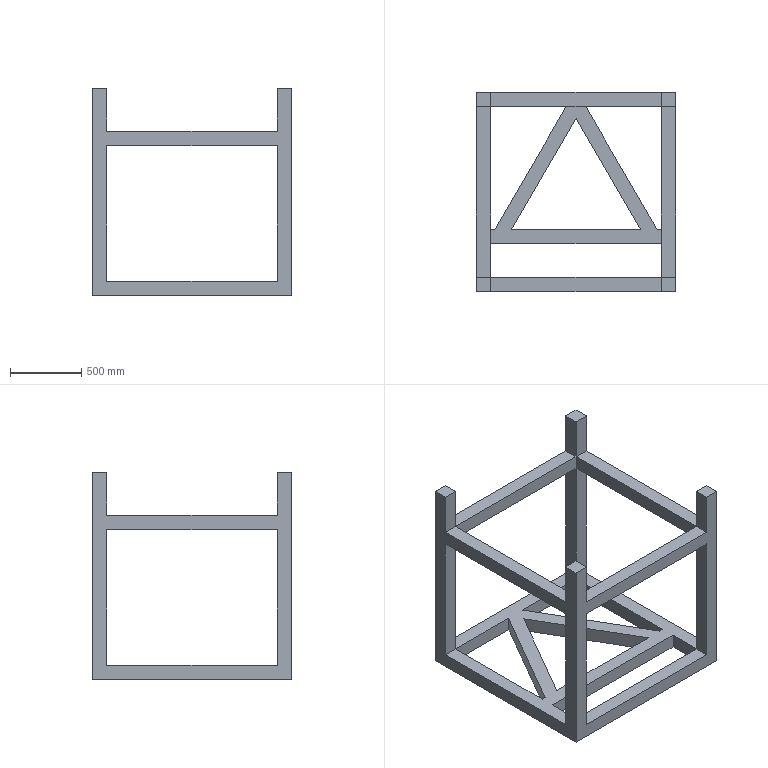Part | SolidWorks | features ICE 3, Extrusion 1 | 1 solid | 54 faces | box 1395 x 1395 x 1450 mm | volume 185057639 mm3 | plane 54
STEP:
#1=CARTESIAN_POINT('',(1395.,1295.,1150.));
#2=VERTEX_POINT('',#1);
#3=CARTESIAN_POINT('',(1295.,1295.,1150.));
#4=VERTEX_POINT('',#3);
#5=CARTESIAN_POINT('',(0.,1295.,1150.));
#6=DIRECTION('',(-1.,0.,0.));
#7=VECTOR('',#6,1000.);
#8=LINE('',#5,#7);
#9=EDGE_CURVE('',#2,#4,#8,.T.);
#10=ORIENTED_EDGE('',*,*,#9,.F.);
#11=CARTESIAN_POINT('',(1395.,1295.,1450.));
#12=VERTEX_POINT('',#11);
#13=CARTESIAN_POINT('',(1395.,1295.,1450.));
#14=DIRECTION('',(0.,0.,-1.));
#15=VECTOR('',#14,1000.);
#16=LINE('',#13,#15);
#17=EDGE_CURVE('',#12,#2,#16,.T.);
#18=ORIENTED_EDGE('',*,*,#17,.F.);
#19=CARTESIAN_POINT('',(1295.,1295.,1450.));
#20=VERTEX_POINT('',#19);
#21=CARTESIAN_POINT('',(1395.,1295.,1450.));
#22=DIRECTION('',(1.,0.,0.));
#23=VECTOR('',#22,1000.);
#24=LINE('',#21,#23);
#25=EDGE_CURVE('',#20,#12,#24,.T.);
#26=ORIENTED_EDGE('',*,*,#25,.F.);
#27=CARTESIAN_POINT('',(1295.,1295.,1450.));
#28=DIRECTION('',(0.,0.,-1.));
#29=VECTOR('',#28,1000.);
#30=LINE('',#27,#29);
#31=EDGE_CURVE('',#20,#4,#30,.T.);
#32=ORIENTED_EDGE('',*,*,#31,.T.);
#33=EDGE_LOOP('',(#10,#18,#26,#32));
#34=FACE_OUTER_BOUND('',#33,.T.);
#35=CARTESIAN_POINT('',(0.,1295.,1450.));
#36=DIRECTION('',(0.,1.,0.));
#37=DIRECTION('',(0.,0.,1.));
#38=AXIS2_PLACEMENT_3D('',#35,#36,#37);
#39=PLANE('',#38);
#40=ADVANCED_FACE('',(#34),#39,.F.);
#41=CARTESIAN_POINT('',(1295.,1295.,1050.));
#42=VERTEX_POINT('',#41);
#43=CARTESIAN_POINT('',(1295.,1295.,1450.));
#44=DIRECTION('',(0.,0.,-1.));
#45=VECTOR('',#44,1000.);
#46=LINE('',#43,#45);
#47=EDGE_CURVE('',#4,#42,#46,.T.);
#48=ORIENTED_EDGE('',*,*,#47,.F.);
#49=CARTESIAN_POINT('',(100.,1295.,1150.));
#50=VERTEX_POINT('',#49);
#51=CARTESIAN_POINT('',(1300.,1295.,1150.));
#52=DIRECTION('',(-1.,0.,0.));
#53=VECTOR('',#52,1000.);
#54=LINE('',#51,#53);
#55=EDGE_CURVE('',#4,#50,#54,.T.);
#56=ORIENTED_EDGE('',*,*,#55,.T.);
#57=CARTESIAN_POINT('',(100.,1295.,1050.));
#58=VERTEX_POINT('',#57);
#59=CARTESIAN_POINT('',(100.,1295.,1450.));
#60=DIRECTION('',(0.,0.,1.));
#61=VECTOR('',#60,1000.);
#62=LINE('',#59,#61);
#63=EDGE_CURVE('',#58,#50,#62,.T.);
#64=ORIENTED_EDGE('',*,*,#63,.F.);
#65=CARTESIAN_POINT('',(1300.,1295.,1050.));
#66=DIRECTION('',(-1.,0.,0.));
#67=VECTOR('',#66,1000.);
#68=LINE('',#65,#67);
#69=EDGE_CURVE('',#42,#58,#68,.T.);
#70=ORIENTED_EDGE('',*,*,#69,.F.);
#71=EDGE_LOOP('',(#48,#56,#64,#70));
#72=FACE_OUTER_BOUND('',#71,.T.);
#73=CARTESIAN_POINT('',(0.,1295.,1450.));
#74=DIRECTION('',(0.,1.,0.));
#75=DIRECTION('',(0.,0.,1.));
#76=AXIS2_PLACEMENT_3D('',#73,#74,#75);
#77=PLANE('',#76);
#78=ADVANCED_FACE('',(#72),#77,.F.);
#79=CARTESIAN_POINT('',(1395.,1295.,1050.));
#80=VERTEX_POINT('',#79);
#81=CARTESIAN_POINT('',(0.,1295.,1050.));
#82=DIRECTION('',(1.,0.,0.));
#83=VECTOR('',#82,1000.);
#84=LINE('',#81,#83);
#85=EDGE_CURVE('',#42,#80,#84,.T.);
#86=ORIENTED_EDGE('',*,*,#85,.F.);
#87=CARTESIAN_POINT('',(1295.,1295.,100.));
#88=VERTEX_POINT('',#87);
#89=CARTESIAN_POINT('',(1295.,1295.,1450.));
#90=DIRECTION('',(0.,0.,-1.));
#91=VECTOR('',#90,1000.);
#92=LINE('',#89,#91);
#93=EDGE_CURVE('',#42,#88,#92,.T.);
#94=ORIENTED_EDGE('',*,*,#93,.T.);
#95=CARTESIAN_POINT('',(1395.,1295.,100.));
#96=VERTEX_POINT('',#95);
#97=CARTESIAN_POINT('',(1395.,1295.,100.));
#98=DIRECTION('',(1.,0.,0.));
#99=VECTOR('',#98,1000.);
#100=LINE('',#97,#99);
#101=EDGE_CURVE('',#88,#96,#100,.T.);
#102=ORIENTED_EDGE('',*,*,#101,.T.);
#103=CARTESIAN_POINT('',(1395.,1295.,1450.));
#104=DIRECTION('',(0.,0.,-1.));
#105=VECTOR('',#104,1000.);
#106=LINE('',#103,#105);
#107=EDGE_CURVE('',#80,#96,#106,.T.);
#108=ORIENTED_EDGE('',*,*,#107,.F.);
#109=EDGE_LOOP('',(#86,#94,#102,#108));
#110=FACE_OUTER_BOUND('',#109,.T.);
#111=CARTESIAN_POINT('',(0.,1295.,1450.));
#112=DIRECTION('',(0.,1.,0.));
#113=DIRECTION('',(0.,0.,1.));
#114=AXIS2_PLACEMENT_3D('',#111,#112,#113);
#115=PLANE('',#114);
#116=ADVANCED_FACE('',(#110),#115,.F.);
#117=CARTESIAN_POINT('',(1295.,100.,1150.));
#118=VERTEX_POINT('',#117);
#119=CARTESIAN_POINT('',(1395.,100.,1150.));
#120=VERTEX_POINT('',#119);
#121=CARTESIAN_POINT('',(1295.,100.,1150.));
#122=DIRECTION('',(1.,0.,0.));
#123=VECTOR('',#122,1000.);
#124=LINE('',#121,#123);
#125=EDGE_CURVE('',#118,#120,#124,.T.);
#126=ORIENTED_EDGE('',*,*,#125,.F.);
#127=CARTESIAN_POINT('',(1295.,100.,1450.));
#128=VERTEX_POINT('',#127);
#129=CARTESIAN_POINT('',(1295.,100.,1450.));
#130=DIRECTION('',(0.,0.,-1.));
#131=VECTOR('',#130,1000.);
#132=LINE('',#129,#131);
#133=EDGE_CURVE('',#128,#118,#132,.T.);
#134=ORIENTED_EDGE('',*,*,#133,.F.);
#135=CARTESIAN_POINT('',(1395.,100.,1450.));
#136=VERTEX_POINT('',#135);
#137=CARTESIAN_POINT('',(1395.,100.,1450.));
#138=DIRECTION('',(-1.,0.,0.));
#139=VECTOR('',#138,1000.);
#140=LINE('',#137,#139);
#141=EDGE_CURVE('',#136,#128,#140,.T.);
#142=ORIENTED_EDGE('',*,*,#141,.F.);
#143=CARTESIAN_POINT('',(1395.,100.,1450.));
#144=DIRECTION('',(0.,0.,-1.));
#145=VECTOR('',#144,1000.);
#146=LINE('',#143,#145);
#147=EDGE_CURVE('',#136,#120,#146,.T.);
#148=ORIENTED_EDGE('',*,*,#147,.T.);
#149=EDGE_LOOP('',(#126,#134,#142,#148));
#150=FACE_OUTER_BOUND('',#149,.T.);
#151=CARTESIAN_POINT('',(0.,100.,1450.));
#152=DIRECTION('',(0.,-1.,0.));
#153=DIRECTION('',(0.,0.,-1.));
#154=AXIS2_PLACEMENT_3D('',#151,#152,#153);
#155=PLANE('',#154);
#156=ADVANCED_FACE('',(#150),#155,.F.);
#157=CARTESIAN_POINT('',(1295.,100.,1050.));
#158=VERTEX_POINT('',#157);
#159=CARTESIAN_POINT('',(1295.,100.,1050.));
#160=DIRECTION('',(0.,0.,1.));
#161=VECTOR('',#160,1000.);
#162=LINE('',#159,#161);
#163=EDGE_CURVE('',#158,#118,#162,.T.);
#164=ORIENTED_EDGE('',*,*,#163,.F.);
#165=CARTESIAN_POINT('',(100.,100.,1050.));
#166=VERTEX_POINT('',#165);
#167=CARTESIAN_POINT('',(1300.,100.,1050.));
#168=DIRECTION('',(-1.,0.,0.));
#169=VECTOR('',#168,1000.);
#170=LINE('',#167,#169);
#171=EDGE_CURVE('',#158,#166,#170,.T.);
#172=ORIENTED_EDGE('',*,*,#171,.T.);
#173=CARTESIAN_POINT('',(100.,100.,1150.));
#174=VERTEX_POINT('',#173);
#175=CARTESIAN_POINT('',(100.,100.,1050.));
#176=DIRECTION('',(0.,0.,-1.));
#177=VECTOR('',#176,1000.);
#178=LINE('',#175,#177);
#179=EDGE_CURVE('',#174,#166,#178,.T.);
#180=ORIENTED_EDGE('',*,*,#179,.F.);
#181=CARTESIAN_POINT('',(1300.,100.,1150.));
#182=DIRECTION('',(-1.,0.,0.));
#183=VECTOR('',#182,1000.);
#184=LINE('',#181,#183);
#185=EDGE_CURVE('',#118,#174,#184,.T.);
#186=ORIENTED_EDGE('',*,*,#185,.F.);
#187=EDGE_LOOP('',(#164,#172,#180,#186));
#188=FACE_OUTER_BOUND('',#187,.T.);
#189=CARTESIAN_POINT('',(0.,100.,1450.));
#190=DIRECTION('',(0.,-1.,0.));
#191=DIRECTION('',(0.,0.,-1.));
#192=AXIS2_PLACEMENT_3D('',#189,#190,#191);
#193=PLANE('',#192);
#194=ADVANCED_FACE('',(#188),#193,.F.);
#195=CARTESIAN_POINT('',(1395.,100.,1050.));
#196=VERTEX_POINT('',#195);
#197=CARTESIAN_POINT('',(1295.,100.,1050.));
#198=DIRECTION('',(-1.,0.,0.));
#199=VECTOR('',#198,1000.);
#200=LINE('',#197,#199);
#201=EDGE_CURVE('',#196,#158,#200,.T.);
#202=ORIENTED_EDGE('',*,*,#201,.F.);
#203=CARTESIAN_POINT('',(1395.,100.,100.));
#204=VERTEX_POINT('',#203);
#205=CARTESIAN_POINT('',(1395.,100.,1450.));
#206=DIRECTION('',(0.,0.,-1.));
#207=VECTOR('',#206,1000.);
#208=LINE('',#205,#207);
#209=EDGE_CURVE('',#196,#204,#208,.T.);
#210=ORIENTED_EDGE('',*,*,#209,.T.);
#211=CARTESIAN_POINT('',(1295.,100.,100.));
#212=VERTEX_POINT('',#211);
#213=CARTESIAN_POINT('',(1395.,100.,100.));
#214=DIRECTION('',(-1.,0.,0.));
#215=VECTOR('',#214,1000.);
#216=LINE('',#213,#215);
#217=EDGE_CURVE('',#204,#212,#216,.T.);
#218=ORIENTED_EDGE('',*,*,#217,.T.);
#219=CARTESIAN_POINT('',(1295.,100.,1450.));
#220=DIRECTION('',(0.,0.,-1.));
#221=VECTOR('',#220,1000.);
#222=LINE('',#219,#221);
#223=EDGE_CURVE('',#158,#212,#222,.T.);
#224=ORIENTED_EDGE('',*,*,#223,.F.);
#225=EDGE_LOOP('',(#202,#210,#218,#224));
#226=FACE_OUTER_BOUND('',#225,.T.);
#227=CARTESIAN_POINT('',(0.,100.,1450.));
#228=DIRECTION('',(0.,-1.,0.));
#229=DIRECTION('',(0.,0.,-1.));
#230=AXIS2_PLACEMENT_3D('',#227,#228,#229);
#231=PLANE('',#230);
#232=ADVANCED_FACE('',(#226),#231,.F.);
#233=CARTESIAN_POINT('',(0.,1295.,1050.));
#234=VERTEX_POINT('',#233);
#235=CARTESIAN_POINT('',(0.,1295.,1050.));
#236=DIRECTION('',(1.,0.,0.));
#237=VECTOR('',#236,1000.);
#238=LINE('',#235,#237);
#239=EDGE_CURVE('',#234,#58,#238,.T.);
#240=ORIENTED_EDGE('',*,*,#239,.F.);
#241=CARTESIAN_POINT('',(0.,1295.,100.));
#242=VERTEX_POINT('',#241);
#243=CARTESIAN_POINT('',(0.,1295.,1450.));
#244=DIRECTION('',(0.,0.,-1.));
#245=VECTOR('',#244,1000.);
#246=LINE('',#243,#245);
#247=EDGE_CURVE('',#234,#242,#246,.T.);
#248=ORIENTED_EDGE('',*,*,#247,.T.);
#249=CARTESIAN_POINT('',(100.,1295.,100.));
#250=VERTEX_POINT('',#249);
#251=CARTESIAN_POINT('',(0.,1295.,100.));
#252=DIRECTION('',(1.,0.,0.));
#253=VECTOR('',#252,1000.);
#254=LINE('',#251,#253);
#255=EDGE_CURVE('',#242,#250,#254,.T.);
#256=ORIENTED_EDGE('',*,*,#255,.T.);
#257=CARTESIAN_POINT('',(100.,1295.,1450.));
#258=DIRECTION('',(0.,0.,-1.));
#259=VECTOR('',#258,1000.);
#260=LINE('',#257,#259);
#261=EDGE_CURVE('',#58,#250,#260,.T.);
#262=ORIENTED_EDGE('',*,*,#261,.F.);
#263=EDGE_LOOP('',(#240,#248,#256,#262));
#264=FACE_OUTER_BOUND('',#263,.T.);
#265=CARTESIAN_POINT('',(0.,1295.,1450.));
#266=DIRECTION('',(0.,1.,0.));
#267=DIRECTION('',(0.,0.,1.));
#268=AXIS2_PLACEMENT_3D('',#265,#266,#267);
#269=PLANE('',#268);
#270=ADVANCED_FACE('',(#264),#269,.F.);
#271=CARTESIAN_POINT('',(0.,1295.,1150.));
#272=VERTEX_POINT('',#271);
#273=CARTESIAN_POINT('',(0.,1295.,1150.));
#274=DIRECTION('',(-1.,0.,0.));
#275=VECTOR('',#274,1000.);
#276=LINE('',#273,#275);
#277=EDGE_CURVE('',#50,#272,#276,.T.);
#278=ORIENTED_EDGE('',*,*,#277,.F.);
#279=CARTESIAN_POINT('',(100.,1295.,1450.));
#280=VERTEX_POINT('',#279);
#281=CARTESIAN_POINT('',(100.,1295.,1450.));
#282=DIRECTION('',(0.,0.,-1.));
#283=VECTOR('',#282,1000.);
#284=LINE('',#281,#283);
#285=EDGE_CURVE('',#280,#50,#284,.T.);
#286=ORIENTED_EDGE('',*,*,#285,.F.);
#287=CARTESIAN_POINT('',(0.,1295.,1450.));
#288=VERTEX_POINT('',#287);
#289=CARTESIAN_POINT('',(0.,1295.,1450.));
#290=DIRECTION('',(1.,0.,0.));
#291=VECTOR('',#290,1000.);
#292=LINE('',#289,#291);
#293=EDGE_CURVE('',#288,#280,#292,.T.);
#294=ORIENTED_EDGE('',*,*,#293,.F.);
#295=CARTESIAN_POINT('',(0.,1295.,1450.));
#296=DIRECTION('',(0.,0.,-1.));
#297=VECTOR('',#296,1000.);
#298=LINE('',#295,#297);
#299=EDGE_CURVE('',#288,#272,#298,.T.);
#300=ORIENTED_EDGE('',*,*,#299,.T.);
#301=EDGE_LOOP('',(#278,#286,#294,#300));
#302=FACE_OUTER_BOUND('',#301,.T.);
#303=CARTESIAN_POINT('',(0.,1295.,1450.));
#304=DIRECTION('',(0.,1.,0.));
#305=DIRECTION('',(0.,0.,1.));
#306=AXIS2_PLACEMENT_3D('',#303,#304,#305);
#307=PLANE('',#306);
#308=ADVANCED_FACE('',(#302),#307,.F.);
#309=CARTESIAN_POINT('',(0.,100.,1050.));
#310=VERTEX_POINT('',#309);
#311=CARTESIAN_POINT('',(100.,100.,1050.));
#312=DIRECTION('',(-1.,0.,0.));
#313=VECTOR('',#312,1000.);
#314=LINE('',#311,#313);
#315=EDGE_CURVE('',#166,#310,#314,.T.);
#316=ORIENTED_EDGE('',*,*,#315,.F.);
#317=CARTESIAN_POINT('',(100.,100.,100.));
#318=VERTEX_POINT('',#317);
#319=CARTESIAN_POINT('',(100.,100.,1450.));
#320=DIRECTION('',(0.,0.,-1.));
#321=VECTOR('',#320,1000.);
#322=LINE('',#319,#321);
#323=EDGE_CURVE('',#166,#318,#322,.T.);
#324=ORIENTED_EDGE('',*,*,#323,.T.);
#325=CARTESIAN_POINT('',(0.,100.,100.));
#326=VERTEX_POINT('',#325);
#327=CARTESIAN_POINT('',(0.,100.,100.));
#328=DIRECTION('',(-1.,0.,0.));
#329=VECTOR('',#328,1000.);
#330=LINE('',#327,#329);
#331=EDGE_CURVE('',#318,#326,#330,.T.);
#332=ORIENTED_EDGE('',*,*,#331,.T.);
#333=CARTESIAN_POINT('',(0.,100.,1450.));
#334=DIRECTION('',(0.,0.,-1.));
#335=VECTOR('',#334,1000.);
#336=LINE('',#333,#335);
#337=EDGE_CURVE('',#310,#326,#336,.T.);
#338=ORIENTED_EDGE('',*,*,#337,.F.);
#339=EDGE_LOOP('',(#316,#324,#332,#338));
#340=FACE_OUTER_BOUND('',#339,.T.);
#341=CARTESIAN_POINT('',(0.,100.,1450.));
#342=DIRECTION('',(0.,-1.,0.));
#343=DIRECTION('',(0.,0.,-1.));
#344=AXIS2_PLACEMENT_3D('',#341,#342,#343);
#345=PLANE('',#344);
#346=ADVANCED_FACE('',(#340),#345,.F.);
#347=CARTESIAN_POINT('',(0.,100.,1150.));
#348=VERTEX_POINT('',#347);
#349=CARTESIAN_POINT('',(100.,100.,1150.));
#350=DIRECTION('',(1.,0.,0.));
#351=VECTOR('',#350,1000.);
#352=LINE('',#349,#351);
#353=EDGE_CURVE('',#348,#174,#352,.T.);
#354=ORIENTED_EDGE('',*,*,#353,.F.);
#355=CARTESIAN_POINT('',(0.,100.,1450.));
#356=VERTEX_POINT('',#355);
#357=CARTESIAN_POINT('',(0.,100.,1450.));
#358=DIRECTION('',(0.,0.,-1.));
#359=VECTOR('',#358,1000.);
#360=LINE('',#357,#359);
#361=EDGE_CURVE('',#356,#348,#360,.T.);
#362=ORIENTED_EDGE('',*,*,#361,.F.);
#363=CARTESIAN_POINT('',(100.,100.,1450.));
#364=VERTEX_POINT('',#363);
#365=CARTESIAN_POINT('',(0.,100.,1450.));
#366=DIRECTION('',(-1.,0.,0.));
#367=VECTOR('',#366,1000.);
#368=LINE('',#365,#367);
#369=EDGE_CURVE('',#364,#356,#368,.T.);
#370=ORIENTED_EDGE('',*,*,#369,.F.);
#371=CARTESIAN_POINT('',(100.,100.,1450.));
#372=DIRECTION('',(0.,0.,-1.));
#373=VECTOR('',#372,1000.);
#374=LINE('',#371,#373);
#375=EDGE_CURVE('',#364,#174,#374,.T.);
#376=ORIENTED_EDGE('',*,*,#375,.T.);
#377=EDGE_LOOP('',(#354,#362,#370,#376));
#378=FACE_OUTER_BOUND('',#377,.T.);
#379=CARTESIAN_POINT('',(0.,100.,1450.));
#380=DIRECTION('',(0.,-1.,0.));
#381=DIRECTION('',(0.,0.,-1.));
#382=AXIS2_PLACEMENT_3D('',#379,#380,#381);
#383=PLANE('',#382);
#384=ADVANCED_FACE('',(#378),#383,.F.);
#385=CARTESIAN_POINT('',(100.,1395.,1050.));
#386=VERTEX_POINT('',#385);
#387=CARTESIAN_POINT('',(100.,1295.,1050.));
#388=DIRECTION('',(0.,1.,0.));
#389=VECTOR('',#388,1000.);
#390=LINE('',#387,#389);
#391=EDGE_CURVE('',#58,#386,#390,.T.);
#392=ORIENTED_EDGE('',*,*,#391,.F.);
#393=ORIENTED_EDGE('',*,*,#261,.T.);
#394=CARTESIAN_POINT('',(100.,1395.,100.));
#395=VERTEX_POINT('',#394);
#396=CARTESIAN_POINT('',(100.,1395.,100.));
#397=DIRECTION('',(0.,1.,0.));
#398=VECTOR('',#397,1000.);
#399=LINE('',#396,#398);
#400=EDGE_CURVE('',#250,#395,#399,.T.);
#401=ORIENTED_EDGE('',*,*,#400,.T.);
#402=CARTESIAN_POINT('',(100.,1395.,1450.));
#403=DIRECTION('',(0.,0.,-1.));
#404=VECTOR('',#403,1000.);
#405=LINE('',#402,#404);
#406=EDGE_CURVE('',#386,#395,#405,.T.);
#407=ORIENTED_EDGE('',*,*,#406,.F.);
#408=EDGE_LOOP('',(#392,#393,#401,#407));
#409=FACE_OUTER_BOUND('',#408,.T.);
#410=CARTESIAN_POINT('',(100.,1395.,1450.));
#411=DIRECTION('',(-1.,0.,0.));
#412=DIRECTION('',(0.,0.,1.));
#413=AXIS2_PLACEMENT_3D('',#410,#411,#412);
#414=PLANE('',#413);
#415=ADVANCED_FACE('',(#409),#414,.F.);
#416=CARTESIAN_POINT('',(100.,1395.,1150.));
#417=VERTEX_POINT('',#416);
#418=CARTESIAN_POINT('',(100.,1295.,1150.));
#419=DIRECTION('',(0.,-1.,0.));
#420=VECTOR('',#419,1000.);
#421=LINE('',#418,#420);
#422=EDGE_CURVE('',#417,#50,#421,.T.);
#423=ORIENTED_EDGE('',*,*,#422,.F.);
#424=CARTESIAN_POINT('',(100.,1395.,1450.));
#425=VERTEX_POINT('',#424);
#426=CARTESIAN_POINT('',(100.,1395.,1450.));
#427=DIRECTION('',(0.,0.,-1.));
#428=VECTOR('',#427,1000.);
#429=LINE('',#426,#428);
#430=EDGE_CURVE('',#425,#417,#429,.T.);
#431=ORIENTED_EDGE('',*,*,#430,.F.);
#432=CARTESIAN_POINT('',(100.,1395.,1450.));
#433=DIRECTION('',(0.,1.,0.));
#434=VECTOR('',#433,1000.);
#435=LINE('',#432,#434);
#436=EDGE_CURVE('',#280,#425,#435,.T.);
#437=ORIENTED_EDGE('',*,*,#436,.F.);
#438=ORIENTED_EDGE('',*,*,#285,.T.);
#439=EDGE_LOOP('',(#423,#431,#437,#438));
#440=FACE_OUTER_BOUND('',#439,.T.);
#441=CARTESIAN_POINT('',(100.,1395.,1450.));
#442=DIRECTION('',(-1.,0.,0.));
#443=DIRECTION('',(0.,0.,1.));
#444=AXIS2_PLACEMENT_3D('',#441,#442,#443);
#445=PLANE('',#444);
#446=ADVANCED_FACE('',(#440),#445,.F.);
#447=CARTESIAN_POINT('',(1295.,1395.,1050.));
#448=VERTEX_POINT('',#447);
#449=CARTESIAN_POINT('',(1295.,1395.,1050.));
#450=DIRECTION('',(0.,-1.,0.));
#451=VECTOR('',#450,1000.);
#452=LINE('',#449,#451);
#453=EDGE_CURVE('',#448,#42,#452,.T.);
#454=ORIENTED_EDGE('',*,*,#453,.F.);
#455=CARTESIAN_POINT('',(1295.,1395.,100.));
#456=VERTEX_POINT('',#455);
#457=CARTESIAN_POINT('',(1295.,1395.,1450.));
#458=DIRECTION('',(0.,0.,-1.));
#459=VECTOR('',#458,1000.);
#460=LINE('',#457,#459);
#461=EDGE_CURVE('',#448,#456,#460,.T.);
#462=ORIENTED_EDGE('',*,*,#461,.T.);
#463=CARTESIAN_POINT('',(1295.,1395.,100.));
#464=DIRECTION('',(0.,-1.,0.));
#465=VECTOR('',#464,1000.);
#466=LINE('',#463,#465);
#467=EDGE_CURVE('',#456,#88,#466,.T.);
#468=ORIENTED_EDGE('',*,*,#467,.T.);
#469=ORIENTED_EDGE('',*,*,#93,.F.);
#470=EDGE_LOOP('',(#454,#462,#468,#469));
#471=FACE_OUTER_BOUND('',#470,.T.);
#472=CARTESIAN_POINT('',(1295.,1395.,1450.));
#473=DIRECTION('',(1.,0.,0.));
#474=DIRECTION('',(0.,0.,-1.));
#475=AXIS2_PLACEMENT_3D('',#472,#473,#474);
#476=PLANE('',#475);
#477=ADVANCED_FACE('',(#471),#476,.F.);
#478=CARTESIAN_POINT('',(1295.,1395.,1150.));
#479=VERTEX_POINT('',#478);
#480=CARTESIAN_POINT('',(1295.,1395.,1150.));
#481=DIRECTION('',(0.,1.,0.));
#482=VECTOR('',#481,1000.);
#483=LINE('',#480,#482);
#484=EDGE_CURVE('',#4,#479,#483,.T.);
#485=ORIENTED_EDGE('',*,*,#484,.F.);
#486=ORIENTED_EDGE('',*,*,#31,.F.);
#487=CARTESIAN_POINT('',(1295.,1395.,1450.));
#488=VERTEX_POINT('',#487);
#489=CARTESIAN_POINT('',(1295.,1395.,1450.));
#490=DIRECTION('',(0.,-1.,0.));
#491=VECTOR('',#490,1000.);
#492=LINE('',#489,#491);
#493=EDGE_CURVE('',#488,#20,#492,.T.);
#494=ORIENTED_EDGE('',*,*,#493,.F.);
#495=CARTESIAN_POINT('',(1295.,1395.,1450.));
#496=DIRECTION('',(0.,0.,-1.));
#497=VECTOR('',#496,1000.);
#498=LINE('',#495,#497);
#499=EDGE_CURVE('',#488,#479,#498,.T.);
#500=ORIENTED_EDGE('',*,*,#499,.T.);
#501=EDGE_LOOP('',(#485,#486,#494,#500));
#502=FACE_OUTER_BOUND('',#501,.T.);
#503=CARTESIAN_POINT('',(1295.,1395.,1450.));
#504=DIRECTION('',(1.,0.,0.));
#505=DIRECTION('',(0.,0.,-1.));
#506=AXIS2_PLACEMENT_3D('',#503,#504,#505);
#507=PLANE('',#506);
#508=ADVANCED_FACE('',(#502),#507,.F.);
#509=CARTESIAN_POINT('',(100.,0.,1050.));
#510=VERTEX_POINT('',#509);
#511=CARTESIAN_POINT('',(100.,0.,1050.));
#512=DIRECTION('',(0.,1.,0.));
#513=VECTOR('',#512,1000.);
#514=LINE('',#511,#513);
#515=EDGE_CURVE('',#510,#166,#514,.T.);
#516=ORIENTED_EDGE('',*,*,#515,.F.);
#517=CARTESIAN_POINT('',(100.,0.,100.));
#518=VERTEX_POINT('',#517);
#519=CARTESIAN_POINT('',(100.,0.,1450.));
#520=DIRECTION('',(0.,0.,-1.));
#521=VECTOR('',#520,1000.);
#522=LINE('',#519,#521);
#523=EDGE_CURVE('',#510,#518,#522,.T.);
#524=ORIENTED_EDGE('',*,*,#523,.T.);
#525=CARTESIAN_POINT('',(100.,0.,100.));
#526=DIRECTION('',(0.,1.,0.));
#527=VECTOR('',#526,1000.);
#528=LINE('',#525,#527);
#529=EDGE_CURVE('',#518,#318,#528,.T.);
#530=ORIENTED_EDGE('',*,*,#529,.T.);
#531=ORIENTED_EDGE('',*,*,#323,.F.);
#532=EDGE_LOOP('',(#516,#524,#530,#531));
#533=FACE_OUTER_BOUND('',#532,.T.);
#534=CARTESIAN_POINT('',(100.,0.,1450.));
#535=DIRECTION('',(-1.,0.,0.));
#536=DIRECTION('',(0.,0.,1.));
#537=AXIS2_PLACEMENT_3D('',#534,#535,#536);
#538=PLANE('',#537);
#539=ADVANCED_FACE('',(#533),#538,.F.);
#540=CARTESIAN_POINT('',(100.,0.,1150.));
#541=VERTEX_POINT('',#540);
#542=CARTESIAN_POINT('',(100.,0.,1150.));
#543=DIRECTION('',(0.,-1.,0.));
#544=VECTOR('',#543,1000.);
#545=LINE('',#542,#544);
#546=EDGE_CURVE('',#174,#541,#545,.T.);
#547=ORIENTED_EDGE('',*,*,#546,.F.);
#548=ORIENTED_EDGE('',*,*,#375,.F.);
#549=CARTESIAN_POINT('',(100.,0.,1450.));
#550=VERTEX_POINT('',#549);
#551=CARTESIAN_POINT('',(100.,0.,1450.));
#552=DIRECTION('',(0.,1.,0.));
#553=VECTOR('',#552,1000.);
#554=LINE('',#551,#553);
#555=EDGE_CURVE('',#550,#364,#554,.T.);
#556=ORIENTED_EDGE('',*,*,#555,.F.);
#557=CARTESIAN_POINT('',(100.,0.,1450.));
#558=DIRECTION('',(0.,0.,-1.));
#559=VECTOR('',#558,1000.);
#560=LINE('',#557,#559);
#561=EDGE_CURVE('',#550,#541,#560,.T.);
#562=ORIENTED_EDGE('',*,*,#561,.T.);
#563=EDGE_LOOP('',(#547,#548,#556,#562));
#564=FACE_OUTER_BOUND('',#563,.T.);
#565=CARTESIAN_POINT('',(100.,0.,1450.));
#566=DIRECTION('',(-1.,0.,0.));
#567=DIRECTION('',(0.,0.,1.));
#568=AXIS2_PLACEMENT_3D('',#565,#566,#567);
#569=PLANE('',#568);
#570=ADVANCED_FACE('',(#564),#569,.F.);
#571=CARTESIAN_POINT('',(1295.,0.,1050.));
#572=VERTEX_POINT('',#571);
#573=CARTESIAN_POINT('',(1295.,0.,1050.));
#574=DIRECTION('',(0.,-1.,0.));
#575=VECTOR('',#574,1000.);
#576=LINE('',#573,#575);
#577=EDGE_CURVE('',#158,#572,#576,.T.);
#578=ORIENTED_EDGE('',*,*,#577,.F.);
#579=ORIENTED_EDGE('',*,*,#223,.T.);
#580=CARTESIAN_POINT('',(1295.,0.,100.));
#581=VERTEX_POINT('',#580);
#582=CARTESIAN_POINT('',(1295.,0.,100.));
#583=DIRECTION('',(0.,-1.,0.));
#584=VECTOR('',#583,1000.);
#585=LINE('',#582,#584);
#586=EDGE_CURVE('',#212,#581,#585,.T.);
#587=ORIENTED_EDGE('',*,*,#586,.T.);
#588=CARTESIAN_POINT('',(1295.,0.,1450.));
#589=DIRECTION('',(0.,0.,-1.));
#590=VECTOR('',#589,1000.);
#591=LINE('',#588,#590);
#592=EDGE_CURVE('',#572,#581,#591,.T.);
#593=ORIENTED_EDGE('',*,*,#592,.F.);
#594=EDGE_LOOP('',(#578,#579,#587,#593));
#595=FACE_OUTER_BOUND('',#594,.T.);
#596=CARTESIAN_POINT('',(1295.,0.,1450.));
#597=DIRECTION('',(1.,0.,0.));
#598=DIRECTION('',(0.,0.,-1.));
#599=AXIS2_PLACEMENT_3D('',#596,#597,#598);
#600=PLANE('',#599);
#601=ADVANCED_FACE('',(#595),#600,.F.);
#602=CARTESIAN_POINT('',(1295.,0.,1150.));
#603=VERTEX_POINT('',#602);
#604=CARTESIAN_POINT('',(1295.,0.,1150.));
#605=DIRECTION('',(0.,1.,0.));
#606=VECTOR('',#605,1000.);
#607=LINE('',#604,#606);
#608=EDGE_CURVE('',#603,#118,#607,.T.);
#609=ORIENTED_EDGE('',*,*,#608,.F.);
#610=CARTESIAN_POINT('',(1295.,0.,1450.));
#611=VERTEX_POINT('',#610);
#612=CARTESIAN_POINT('',(1295.,0.,1450.));
#613=DIRECTION('',(0.,0.,-1.));
#614=VECTOR('',#613,1000.);
#615=LINE('',#612,#614);
#616=EDGE_CURVE('',#611,#603,#615,.T.);
#617=ORIENTED_EDGE('',*,*,#616,.F.);
#618=CARTESIAN_POINT('',(1295.,0.,1450.));
#619=DIRECTION('',(0.,-1.,0.));
#620=VECTOR('',#619,1000.);
#621=LINE('',#618,#620);
#622=EDGE_CURVE('',#128,#611,#621,.T.);
#623=ORIENTED_EDGE('',*,*,#622,.F.);
#624=ORIENTED_EDGE('',*,*,#133,.T.);
#625=EDGE_LOOP('',(#609,#617,#623,#624));
#626=FACE_OUTER_BOUND('',#625,.T.);
#627=CARTESIAN_POINT('',(1295.,0.,1450.));
#628=DIRECTION('',(1.,0.,0.));
#629=DIRECTION('',(0.,0.,-1.));
#630=AXIS2_PLACEMENT_3D('',#627,#628,#629);
#631=PLANE('',#630);
#632=ADVANCED_FACE('',(#626),#631,.F.);
#633=CARTESIAN_POINT('',(697.5,1215.,100.));
#634=VERTEX_POINT('',#633);
#635=CARTESIAN_POINT('',(245.572,435.,100.));
#636=VERTEX_POINT('',#635);
#637=CARTESIAN_POINT('',(697.5,1215.,100.));
#638=DIRECTION('',(-0.5013,-0.8653,0.));
#639=VECTOR('',#638,1000.);
#640=LINE('',#637,#639);
#641=EDGE_CURVE('',#634,#636,#640,.T.);
#642=ORIENTED_EDGE('',*,*,#641,.F.);
#643=CARTESIAN_POINT('',(1149.428,435.,100.));
#644=VERTEX_POINT('',#643);
#645=CARTESIAN_POINT('',(697.5,1215.,100.));
#646=DIRECTION('',(-0.5013,0.8653,0.));
#647=VECTOR('',#646,1000.);
#648=LINE('',#645,#647);
#649=EDGE_CURVE('',#644,#634,#648,.T.);
#650=ORIENTED_EDGE('',*,*,#649,.F.);
#651=CARTESIAN_POINT('',(245.572,435.,100.));
#652=DIRECTION('',(1.,0.,0.));
#653=VECTOR('',#652,1000.);
#654=LINE('',#651,#653);
#655=EDGE_CURVE('',#636,#644,#654,.T.);
#656=ORIENTED_EDGE('',*,*,#655,.F.);
#657=EDGE_LOOP('',(#642,#650,#656));
#658=FACE_BOUND('',#657,.T.);
#659=ORIENTED_EDGE('',*,*,#217,.F.);
#660=CARTESIAN_POINT('',(1395.,0.,100.));
#661=DIRECTION('',(0.,1.,0.));
#662=VECTOR('',#661,1000.);
#663=LINE('',#660,#662);
#664=EDGE_CURVE('',#204,#96,#663,.T.);
#665=ORIENTED_EDGE('',*,*,#664,.T.);
#666=ORIENTED_EDGE('',*,*,#101,.F.);
#667=CARTESIAN_POINT('',(1295.,435.,100.));
#668=VERTEX_POINT('',#667);
#669=CARTESIAN_POINT('',(1295.,435.,100.));
#670=DIRECTION('',(0.,1.,0.));
#671=VECTOR('',#670,1000.);
#672=LINE('',#669,#671);
#673=EDGE_CURVE('',#668,#88,#672,.T.);
#674=ORIENTED_EDGE('',*,*,#673,.F.);
#675=CARTESIAN_POINT('',(1265.,435.,100.));
#676=VERTEX_POINT('',#675);
#677=CARTESIAN_POINT('',(1265.,435.,100.));
#678=DIRECTION('',(1.,0.,0.));
#679=VECTOR('',#678,1000.);
#680=LINE('',#677,#679);
#681=EDGE_CURVE('',#676,#668,#680,.T.);
#682=ORIENTED_EDGE('',*,*,#681,.F.);
#683=CARTESIAN_POINT('',(766.721,1295.,100.));
#684=VERTEX_POINT('',#683);
#685=CARTESIAN_POINT('',(766.721,1295.,100.));
#686=DIRECTION('',(0.5013,-0.8653,0.));
#687=VECTOR('',#686,1000.);
#688=LINE('',#685,#687);
#689=EDGE_CURVE('',#684,#676,#688,.T.);
#690=ORIENTED_EDGE('',*,*,#689,.F.);
#691=CARTESIAN_POINT('',(766.721,1295.,100.));
#692=DIRECTION('',(-1.,0.,0.));
#693=VECTOR('',#692,1000.);
#694=LINE('',#691,#693);
#695=EDGE_CURVE('',#88,#684,#694,.T.);
#696=ORIENTED_EDGE('',*,*,#695,.F.);
#697=ORIENTED_EDGE('',*,*,#467,.F.);
#698=CARTESIAN_POINT('',(0.,1395.,100.));
#699=DIRECTION('',(-1.,0.,0.));
#700=VECTOR('',#699,1000.);
#701=LINE('',#698,#700);
#702=EDGE_CURVE('',#456,#395,#701,.T.);
#703=ORIENTED_EDGE('',*,*,#702,.T.);
#704=ORIENTED_EDGE('',*,*,#400,.F.);
#705=CARTESIAN_POINT('',(628.279,1295.,100.));
#706=VERTEX_POINT('',#705);
#707=CARTESIAN_POINT('',(100.,1295.,100.));
#708=DIRECTION('',(-1.,0.,0.));
#709=VECTOR('',#708,1000.);
#710=LINE('',#707,#709);
#711=EDGE_CURVE('',#706,#250,#710,.T.);
#712=ORIENTED_EDGE('',*,*,#711,.F.);
#713=CARTESIAN_POINT('',(130.,435.,100.));
#714=VERTEX_POINT('',#713);
#715=CARTESIAN_POINT('',(628.279,1295.,100.));
#716=DIRECTION('',(0.5013,0.8653,0.));
#717=VECTOR('',#716,1000.);
#718=LINE('',#715,#717);
#719=EDGE_CURVE('',#714,#706,#718,.T.);
#720=ORIENTED_EDGE('',*,*,#719,.F.);
#721=CARTESIAN_POINT('',(100.,435.,100.));
#722=VERTEX_POINT('',#721);
#723=CARTESIAN_POINT('',(100.,435.,100.));
#724=DIRECTION('',(1.,0.,0.));
#725=VECTOR('',#724,1000.);
#726=LINE('',#723,#725);
#727=EDGE_CURVE('',#722,#714,#726,.T.);
#728=ORIENTED_EDGE('',*,*,#727,.F.);
#729=CARTESIAN_POINT('',(100.,435.,100.));
#730=DIRECTION('',(0.,-1.,0.));
#731=VECTOR('',#730,1000.);
#732=LINE('',#729,#731);
#733=EDGE_CURVE('',#250,#722,#732,.T.);
#734=ORIENTED_EDGE('',*,*,#733,.F.);
#735=ORIENTED_EDGE('',*,*,#255,.F.);
#736=CARTESIAN_POINT('',(0.,0.,100.));
#737=DIRECTION('',(0.,-1.,0.));
#738=VECTOR('',#737,1000.);
#739=LINE('',#736,#738);
#740=EDGE_CURVE('',#242,#326,#739,.T.);
#741=ORIENTED_EDGE('',*,*,#740,.T.);
#742=ORIENTED_EDGE('',*,*,#331,.F.);
#743=CARTESIAN_POINT('',(100.,335.,100.));
#744=VERTEX_POINT('',#743);
#745=CARTESIAN_POINT('',(100.,100.,100.));
#746=DIRECTION('',(0.,-1.,0.));
#747=VECTOR('',#746,1000.);
#748=LINE('',#745,#747);
#749=EDGE_CURVE('',#744,#318,#748,.T.);
#750=ORIENTED_EDGE('',*,*,#749,.F.);
#751=CARTESIAN_POINT('',(1295.,335.,100.));
#752=VERTEX_POINT('',#751);
#753=CARTESIAN_POINT('',(100.,335.,100.));
#754=DIRECTION('',(-1.,0.,0.));
#755=VECTOR('',#754,1000.);
#756=LINE('',#753,#755);
#757=EDGE_CURVE('',#752,#744,#756,.T.);
#758=ORIENTED_EDGE('',*,*,#757,.F.);
#759=CARTESIAN_POINT('',(1295.,100.,100.));
#760=DIRECTION('',(0.,1.,0.));
#761=VECTOR('',#760,1000.);
#762=LINE('',#759,#761);
#763=EDGE_CURVE('',#212,#752,#762,.T.);
#764=ORIENTED_EDGE('',*,*,#763,.F.);
#765=EDGE_LOOP('',(#659,#665,#666,#674,#682,#690,#696,#697,#703,#704,#712,#720,#728,#734,#735,#741,#742,#750,#758,#764));
#766=FACE_OUTER_BOUND('',#765,.T.);
#767=CARTESIAN_POINT('',(0.,0.,100.));
#768=DIRECTION('',(0.,0.,-1.));
#769=DIRECTION('',(-1.,0.,0.));
#770=AXIS2_PLACEMENT_3D('',#767,#768,#769);
#771=PLANE('',#770);
#772=ADVANCED_FACE('',(#658,#766),#771,.F.);
#773=ORIENTED_EDGE('',*,*,#586,.F.);
#774=CARTESIAN_POINT('',(100.,100.,100.));
#775=DIRECTION('',(1.,0.,0.));
#776=VECTOR('',#775,1000.);
#777=LINE('',#774,#776);
#778=EDGE_CURVE('',#318,#212,#777,.T.);
#779=ORIENTED_EDGE('',*,*,#778,.F.);
#780=ORIENTED_EDGE('',*,*,#529,.F.);
#781=CARTESIAN_POINT('',(0.,0.,100.));
#782=DIRECTION('',(1.,0.,0.));
#783=VECTOR('',#782,1000.);
#784=LINE('',#781,#783);
#785=EDGE_CURVE('',#518,#581,#784,.T.);
#786=ORIENTED_EDGE('',*,*,#785,.T.);
#787=EDGE_LOOP('',(#773,#779,#780,#786));
#788=FACE_OUTER_BOUND('',#787,.T.);
#789=CARTESIAN_POINT('',(0.,0.,100.));
#790=DIRECTION('',(0.,0.,-1.));
#791=DIRECTION('',(-1.,0.,0.));
#792=AXIS2_PLACEMENT_3D('',#789,#790,#791);
#793=PLANE('',#792);
#794=ADVANCED_FACE('',(#788),#793,.F.);
#795=CARTESIAN_POINT('',(0.,1395.,0.));
#796=VERTEX_POINT('',#795);
#797=CARTESIAN_POINT('',(0.,0.,0.));
#798=VERTEX_POINT('',#797);
#799=CARTESIAN_POINT('',(0.,0.,0.));
#800=DIRECTION('',(0.,-1.,0.));
#801=VECTOR('',#800,1000.);
#802=LINE('',#799,#801);
#803=EDGE_CURVE('',#796,#798,#802,.T.);
#804=ORIENTED_EDGE('',*,*,#803,.F.);
#805=CARTESIAN_POINT('',(1395.,1395.,0.));
#806=VERTEX_POINT('',#805);
#807=CARTESIAN_POINT('',(0.,1395.,0.));
#808=DIRECTION('',(-1.,0.,0.));
#809=VECTOR('',#808,1000.);
#810=LINE('',#807,#809);
#811=EDGE_CURVE('',#806,#796,#810,.T.);
#812=ORIENTED_EDGE('',*,*,#811,.F.);
#813=CARTESIAN_POINT('',(1395.,0.,0.));
#814=VERTEX_POINT('',#813);
#815=CARTESIAN_POINT('',(1395.,0.,0.));
#816=DIRECTION('',(0.,1.,0.));
#817=VECTOR('',#816,1000.);
#818=LINE('',#815,#817);
#819=EDGE_CURVE('',#814,#806,#818,.T.);
#820=ORIENTED_EDGE('',*,*,#819,.F.);
#821=CARTESIAN_POINT('',(0.,0.,0.));
#822=DIRECTION('',(1.,0.,0.));
#823=VECTOR('',#822,1000.);
#824=LINE('',#821,#823);
#825=EDGE_CURVE('',#798,#814,#824,.T.);
#826=ORIENTED_EDGE('',*,*,#825,.F.);
#827=EDGE_LOOP('',(#804,#812,#820,#826));
#828=FACE_OUTER_BOUND('',#827,.T.);
#829=CARTESIAN_POINT('',(100.,335.,0.));
#830=VERTEX_POINT('',#829);
#831=CARTESIAN_POINT('',(100.,100.,0.));
#832=VERTEX_POINT('',#831);
#833=CARTESIAN_POINT('',(100.,100.,0.));
#834=DIRECTION('',(0.,-1.,0.));
#835=VECTOR('',#834,1000.);
#836=LINE('',#833,#835);
#837=EDGE_CURVE('',#830,#832,#836,.T.);
#838=ORIENTED_EDGE('',*,*,#837,.T.);
#839=CARTESIAN_POINT('',(1295.,100.,0.));
#840=VERTEX_POINT('',#839);
#841=CARTESIAN_POINT('',(100.,100.,0.));
#842=DIRECTION('',(1.,0.,0.));
#843=VECTOR('',#842,1000.);
#844=LINE('',#841,#843);
#845=EDGE_CURVE('',#832,#840,#844,.T.);
#846=ORIENTED_EDGE('',*,*,#845,.T.);
#847=CARTESIAN_POINT('',(1295.,335.,0.));
#848=VERTEX_POINT('',#847);
#849=CARTESIAN_POINT('',(1295.,100.,0.));
#850=DIRECTION('',(0.,1.,0.));
#851=VECTOR('',#850,1000.);
#852=LINE('',#849,#851);
#853=EDGE_CURVE('',#840,#848,#852,.T.);
#854=ORIENTED_EDGE('',*,*,#853,.T.);
#855=CARTESIAN_POINT('',(100.,335.,0.));
#856=DIRECTION('',(-1.,0.,0.));
#857=VECTOR('',#856,1000.);
#858=LINE('',#855,#857);
#859=EDGE_CURVE('',#848,#830,#858,.T.);
#860=ORIENTED_EDGE('',*,*,#859,.T.);
#861=EDGE_LOOP('',(#838,#846,#854,#860));
#862=FACE_BOUND('',#861,.T.);
#863=CARTESIAN_POINT('',(628.279,1295.,0.));
#864=VERTEX_POINT('',#863);
#865=CARTESIAN_POINT('',(100.,1295.,0.));
#866=VERTEX_POINT('',#865);
#867=CARTESIAN_POINT('',(100.,1295.,0.));
#868=DIRECTION('',(-1.,0.,0.));
#869=VECTOR('',#868,1000.);
#870=LINE('',#867,#869);
#871=EDGE_CURVE('',#864,#866,#870,.T.);
#872=ORIENTED_EDGE('',*,*,#871,.T.);
#873=CARTESIAN_POINT('',(100.,435.,0.));
#874=VERTEX_POINT('',#873);
#875=CARTESIAN_POINT('',(100.,435.,0.));
#876=DIRECTION('',(0.,-1.,0.));
#877=VECTOR('',#876,1000.);
#878=LINE('',#875,#877);
#879=EDGE_CURVE('',#866,#874,#878,.T.);
#880=ORIENTED_EDGE('',*,*,#879,.T.);
#881=CARTESIAN_POINT('',(130.,435.,0.));
#882=VERTEX_POINT('',#881);
#883=CARTESIAN_POINT('',(100.,435.,0.));
#884=DIRECTION('',(1.,0.,0.));
#885=VECTOR('',#884,1000.);
#886=LINE('',#883,#885);
#887=EDGE_CURVE('',#874,#882,#886,.T.);
#888=ORIENTED_EDGE('',*,*,#887,.T.);
#889=CARTESIAN_POINT('',(628.279,1295.,0.));
#890=DIRECTION('',(0.5013,0.8653,0.));
#891=VECTOR('',#890,1000.);
#892=LINE('',#889,#891);
#893=EDGE_CURVE('',#882,#864,#892,.T.);
#894=ORIENTED_EDGE('',*,*,#893,.T.);
#895=EDGE_LOOP('',(#872,#880,#888,#894));
#896=FACE_BOUND('',#895,.T.);
#897=CARTESIAN_POINT('',(1265.,435.,0.));
#898=VERTEX_POINT('',#897);
#899=CARTESIAN_POINT('',(1295.,435.,0.));
#900=VERTEX_POINT('',#899);
#901=CARTESIAN_POINT('',(1265.,435.,0.));
#902=DIRECTION('',(1.,0.,0.));
#903=VECTOR('',#902,1000.);
#904=LINE('',#901,#903);
#905=EDGE_CURVE('',#898,#900,#904,.T.);
#906=ORIENTED_EDGE('',*,*,#905,.T.);
#907=CARTESIAN_POINT('',(1295.,1295.,0.));
#908=VERTEX_POINT('',#907);
#909=CARTESIAN_POINT('',(1295.,435.,0.));
#910=DIRECTION('',(0.,1.,0.));
#911=VECTOR('',#910,1000.);
#912=LINE('',#909,#911);
#913=EDGE_CURVE('',#900,#908,#912,.T.);
#914=ORIENTED_EDGE('',*,*,#913,.T.);
#915=CARTESIAN_POINT('',(766.721,1295.,0.));
#916=VERTEX_POINT('',#915);
#917=CARTESIAN_POINT('',(766.721,1295.,0.));
#918=DIRECTION('',(-1.,0.,0.));
#919=VECTOR('',#918,1000.);
#920=LINE('',#917,#919);
#921=EDGE_CURVE('',#908,#916,#920,.T.);
#922=ORIENTED_EDGE('',*,*,#921,.T.);
#923=CARTESIAN_POINT('',(766.721,1295.,0.));
#924=DIRECTION('',(0.5013,-0.8653,0.));
#925=VECTOR('',#924,1000.);
#926=LINE('',#923,#925);
#927=EDGE_CURVE('',#916,#898,#926,.T.);
#928=ORIENTED_EDGE('',*,*,#927,.T.);
#929=EDGE_LOOP('',(#906,#914,#922,#928));
#930=FACE_BOUND('',#929,.T.);
#931=CARTESIAN_POINT('',(1149.428,435.,0.));
#932=VERTEX_POINT('',#931);
#933=CARTESIAN_POINT('',(697.5,1215.,0.));
#934=VERTEX_POINT('',#933);
#935=CARTESIAN_POINT('',(697.5,1215.,0.));
#936=DIRECTION('',(-0.5013,0.8653,0.));
#937=VECTOR('',#936,1000.);
#938=LINE('',#935,#937);
#939=EDGE_CURVE('',#932,#934,#938,.T.);
#940=ORIENTED_EDGE('',*,*,#939,.T.);
#941=CARTESIAN_POINT('',(245.572,435.,0.));
#942=VERTEX_POINT('',#941);
#943=CARTESIAN_POINT('',(697.5,1215.,0.));
#944=DIRECTION('',(-0.5013,-0.8653,0.));
#945=VECTOR('',#944,1000.);
#946=LINE('',#943,#945);
#947=EDGE_CURVE('',#934,#942,#946,.T.);
#948=ORIENTED_EDGE('',*,*,#947,.T.);
#949=CARTESIAN_POINT('',(245.572,435.,0.));
#950=DIRECTION('',(1.,0.,0.));
#951=VECTOR('',#950,1000.);
#952=LINE('',#949,#951);
#953=EDGE_CURVE('',#942,#932,#952,.T.);
#954=ORIENTED_EDGE('',*,*,#953,.T.);
#955=EDGE_LOOP('',(#940,#948,#954));
#956=FACE_BOUND('',#955,.T.);
#957=CARTESIAN_POINT('',(0.,0.,0.));
#958=DIRECTION('',(0.,0.,-1.));
#959=DIRECTION('',(-1.,0.,0.));
#960=AXIS2_PLACEMENT_3D('',#957,#958,#959);
#961=PLANE('',#960);
#962=ADVANCED_FACE('',(#828,#862,#896,#930,#956),#961,.T.);
#963=ORIENTED_EDGE('',*,*,#247,.F.);
#964=CARTESIAN_POINT('',(0.,1300.,1050.));
#965=DIRECTION('',(0.,-1.,0.));
#966=VECTOR('',#965,1000.);
#967=LINE('',#964,#966);
#968=EDGE_CURVE('',#234,#310,#967,.T.);
#969=ORIENTED_EDGE('',*,*,#968,.T.);
#970=ORIENTED_EDGE('',*,*,#337,.T.);
#971=ORIENTED_EDGE('',*,*,#740,.F.);
#972=EDGE_LOOP('',(#963,#969,#970,#971));
#973=FACE_BOUND('',#972,.T.);
#974=CARTESIAN_POINT('',(0.,1300.,1150.));
#975=DIRECTION('',(0.,-1.,0.));
#976=VECTOR('',#975,1000.);
#977=LINE('',#974,#976);
#978=EDGE_CURVE('',#272,#348,#977,.T.);
#979=ORIENTED_EDGE('',*,*,#978,.F.);
#980=ORIENTED_EDGE('',*,*,#299,.F.);
#981=CARTESIAN_POINT('',(0.,1395.,1450.));
#982=VERTEX_POINT('',#981);
#983=CARTESIAN_POINT('',(0.,1395.,1450.));
#984=DIRECTION('',(0.,-1.,0.));
#985=VECTOR('',#984,1000.);
#986=LINE('',#983,#985);
#987=EDGE_CURVE('',#982,#288,#986,.T.);
#988=ORIENTED_EDGE('',*,*,#987,.F.);
#989=CARTESIAN_POINT('',(0.,1395.,100.));
#990=DIRECTION('',(0.,0.,-1.));
#991=VECTOR('',#990,1000.);
#992=LINE('',#989,#991);
#993=EDGE_CURVE('',#982,#796,#992,.T.);
#994=ORIENTED_EDGE('',*,*,#993,.T.);
#995=ORIENTED_EDGE('',*,*,#803,.T.);
#996=CARTESIAN_POINT('',(0.,0.,1450.));
#997=VERTEX_POINT('',#996);
#998=CARTESIAN_POINT('',(0.,0.,100.));
#999=DIRECTION('',(0.,0.,-1.));
#1000=VECTOR('',#999,1000.);
#1001=LINE('',#998,#1000);
#1002=EDGE_CURVE('',#997,#798,#1001,.T.);
#1003=ORIENTED_EDGE('',*,*,#1002,.F.);
#1004=CARTESIAN_POINT('',(0.,0.,1450.));
#1005=DIRECTION('',(0.,-1.,0.));
#1006=VECTOR('',#1005,1000.);
#1007=LINE('',#1004,#1006);
#1008=EDGE_CURVE('',#356,#997,#1007,.T.);
#1009=ORIENTED_EDGE('',*,*,#1008,.F.);
#1010=ORIENTED_EDGE('',*,*,#361,.T.);
#1011=EDGE_LOOP('',(#979,#980,#988,#994,#995,#1003,#1009,#1010));
#1012=FACE_OUTER_BOUND('',#1011,.T.);
#1013=CARTESIAN_POINT('',(0.,0.,100.));
#1014=DIRECTION('',(1.,0.,0.));
#1015=DIRECTION('',(0.,0.,-1.));
#1016=AXIS2_PLACEMENT_3D('',#1013,#1014,#1015);
#1017=PLANE('',#1016);
#1018=ADVANCED_FACE('',(#973,#1012),#1017,.F.);
#1019=ORIENTED_EDGE('',*,*,#616,.T.);
#1020=CARTESIAN_POINT('',(1300.,0.,1150.));
#1021=DIRECTION('',(-1.,0.,0.));
#1022=VECTOR('',#1021,1000.);
#1023=LINE('',#1020,#1022);
#1024=EDGE_CURVE('',#603,#541,#1023,.T.);
#1025=ORIENTED_EDGE('',*,*,#1024,.T.);
#1026=ORIENTED_EDGE('',*,*,#561,.F.);
#1027=CARTESIAN_POINT('',(0.,0.,1450.));
#1028=DIRECTION('',(1.,0.,0.));
#1029=VECTOR('',#1028,1000.);
#1030=LINE('',#1027,#1029);
#1031=EDGE_CURVE('',#997,#550,#1030,.T.);
#1032=ORIENTED_EDGE('',*,*,#1031,.F.);
#1033=ORIENTED_EDGE('',*,*,#1002,.T.);
#1034=ORIENTED_EDGE('',*,*,#825,.T.);
#1035=CARTESIAN_POINT('',(1395.,0.,1450.));
#1036=VERTEX_POINT('',#1035);
#1037=CARTESIAN_POINT('',(1395.,0.,100.));
#1038=DIRECTION('',(0.,0.,-1.));
#1039=VECTOR('',#1038,1000.);
#1040=LINE('',#1037,#1039);
#1041=EDGE_CURVE('',#1036,#814,#1040,.T.);
#1042=ORIENTED_EDGE('',*,*,#1041,.F.);
#1043=CARTESIAN_POINT('',(1395.,0.,1450.));
#1044=DIRECTION('',(1.,0.,0.));
#1045=VECTOR('',#1044,1000.);
#1046=LINE('',#1043,#1045);
#1047=EDGE_CURVE('',#611,#1036,#1046,.T.);
#1048=ORIENTED_EDGE('',*,*,#1047,.F.);
#1049=EDGE_LOOP('',(#1019,#1025,#1026,#1032,#1033,#1034,#1042,#1048));
#1050=FACE_OUTER_BOUND('',#1049,.T.);
#1051=CARTESIAN_POINT('',(1300.,0.,1050.));
#1052=DIRECTION('',(-1.,0.,0.));
#1053=VECTOR('',#1052,1000.);
#1054=LINE('',#1051,#1053);
#1055=EDGE_CURVE('',#572,#510,#1054,.T.);
#1056=ORIENTED_EDGE('',*,*,#1055,.F.);
#1057=ORIENTED_EDGE('',*,*,#592,.T.);
#1058=ORIENTED_EDGE('',*,*,#785,.F.);
#1059=ORIENTED_EDGE('',*,*,#523,.F.);
#1060=EDGE_LOOP('',(#1056,#1057,#1058,#1059));
#1061=FACE_BOUND('',#1060,.T.);
#1062=CARTESIAN_POINT('',(0.,0.,100.));
#1063=DIRECTION('',(0.,1.,0.));
#1064=DIRECTION('',(0.,0.,1.));
#1065=AXIS2_PLACEMENT_3D('',#1062,#1063,#1064);
#1066=PLANE('',#1065);
#1067=ADVANCED_FACE('',(#1050,#1061),#1066,.F.);
#1068=CARTESIAN_POINT('',(1395.,1300.,1050.));
#1069=DIRECTION('',(0.,-1.,0.));
#1070=VECTOR('',#1069,1000.);
#1071=LINE('',#1068,#1070);
#1072=EDGE_CURVE('',#80,#196,#1071,.T.);
#1073=ORIENTED_EDGE('',*,*,#1072,.F.);
#1074=ORIENTED_EDGE('',*,*,#107,.T.);
#1075=ORIENTED_EDGE('',*,*,#664,.F.);
#1076=ORIENTED_EDGE('',*,*,#209,.F.);
#1077=EDGE_LOOP('',(#1073,#1074,#1075,#1076));
#1078=FACE_BOUND('',#1077,.T.);
#1079=ORIENTED_EDGE('',*,*,#17,.T.);
#1080=CARTESIAN_POINT('',(1395.,1300.,1150.));
#1081=DIRECTION('',(0.,-1.,0.));
#1082=VECTOR('',#1081,1000.);
#1083=LINE('',#1080,#1082);
#1084=EDGE_CURVE('',#2,#120,#1083,.T.);
#1085=ORIENTED_EDGE('',*,*,#1084,.T.);
#1086=ORIENTED_EDGE('',*,*,#147,.F.);
#1087=CARTESIAN_POINT('',(1395.,0.,1450.));
#1088=DIRECTION('',(0.,1.,0.));
#1089=VECTOR('',#1088,1000.);
#1090=LINE('',#1087,#1089);
#1091=EDGE_CURVE('',#1036,#136,#1090,.T.);
#1092=ORIENTED_EDGE('',*,*,#1091,.F.);
#1093=ORIENTED_EDGE('',*,*,#1041,.T.);
#1094=ORIENTED_EDGE('',*,*,#819,.T.);
#1095=CARTESIAN_POINT('',(1395.,1395.,1450.));
#1096=VERTEX_POINT('',#1095);
#1097=CARTESIAN_POINT('',(1395.,1395.,100.));
#1098=DIRECTION('',(0.,0.,-1.));
#1099=VECTOR('',#1098,1000.);
#1100=LINE('',#1097,#1099);
#1101=EDGE_CURVE('',#1096,#806,#1100,.T.);
#1102=ORIENTED_EDGE('',*,*,#1101,.F.);
#1103=CARTESIAN_POINT('',(1395.,1395.,1450.));
#1104=DIRECTION('',(0.,1.,0.));
#1105=VECTOR('',#1104,1000.);
#1106=LINE('',#1103,#1105);
#1107=EDGE_CURVE('',#12,#1096,#1106,.T.);
#1108=ORIENTED_EDGE('',*,*,#1107,.F.);
#1109=EDGE_LOOP('',(#1079,#1085,#1086,#1092,#1093,#1094,#1102,#1108));
#1110=FACE_OUTER_BOUND('',#1109,.T.);
#1111=CARTESIAN_POINT('',(1395.,0.,100.));
#1112=DIRECTION('',(-1.,0.,0.));
#1113=DIRECTION('',(0.,0.,1.));
#1114=AXIS2_PLACEMENT_3D('',#1111,#1112,#1113);
#1115=PLANE('',#1114);
#1116=ADVANCED_FACE('',(#1078,#1110),#1115,.F.);
#1117=ORIENTED_EDGE('',*,*,#461,.F.);
#1118=CARTESIAN_POINT('',(1300.,1395.,1050.));
#1119=DIRECTION('',(-1.,0.,0.));
#1120=VECTOR('',#1119,1000.);
#1121=LINE('',#1118,#1120);
#1122=EDGE_CURVE('',#448,#386,#1121,.T.);
#1123=ORIENTED_EDGE('',*,*,#1122,.T.);
#1124=ORIENTED_EDGE('',*,*,#406,.T.);
#1125=ORIENTED_EDGE('',*,*,#702,.F.);
#1126=EDGE_LOOP('',(#1117,#1123,#1124,#1125));
#1127=FACE_BOUND('',#1126,.T.);
#1128=CARTESIAN_POINT('',(1300.,1395.,1150.));
#1129=DIRECTION('',(-1.,0.,0.));
#1130=VECTOR('',#1129,1000.);
#1131=LINE('',#1128,#1130);
#1132=EDGE_CURVE('',#479,#417,#1131,.T.);
#1133=ORIENTED_EDGE('',*,*,#1132,.F.);
#1134=ORIENTED_EDGE('',*,*,#499,.F.);
#1135=CARTESIAN_POINT('',(1395.,1395.,1450.));
#1136=DIRECTION('',(-1.,0.,0.));
#1137=VECTOR('',#1136,1000.);
#1138=LINE('',#1135,#1137);
#1139=EDGE_CURVE('',#1096,#488,#1138,.T.);
#1140=ORIENTED_EDGE('',*,*,#1139,.F.);
#1141=ORIENTED_EDGE('',*,*,#1101,.T.);
#1142=ORIENTED_EDGE('',*,*,#811,.T.);
#1143=ORIENTED_EDGE('',*,*,#993,.F.);
#1144=CARTESIAN_POINT('',(0.,1395.,1450.));
#1145=DIRECTION('',(-1.,0.,0.));
#1146=VECTOR('',#1145,1000.);
#1147=LINE('',#1144,#1146);
#1148=EDGE_CURVE('',#425,#982,#1147,.T.);
#1149=ORIENTED_EDGE('',*,*,#1148,.F.);
#1150=ORIENTED_EDGE('',*,*,#430,.T.);
#1151=EDGE_LOOP('',(#1133,#1134,#1140,#1141,#1142,#1143,#1149,#1150));
#1152=FACE_OUTER_BOUND('',#1151,.T.);
#1153=CARTESIAN_POINT('',(0.,1395.,100.));
#1154=DIRECTION('',(0.,-1.,0.));
#1155=DIRECTION('',(0.,0.,-1.));
#1156=AXIS2_PLACEMENT_3D('',#1153,#1154,#1155);
#1157=PLANE('',#1156);
#1158=ADVANCED_FACE('',(#1127,#1152),#1157,.F.);
#1159=ORIENTED_EDGE('',*,*,#845,.F.);
#1160=CARTESIAN_POINT('',(100.,100.,100.));
#1161=DIRECTION('',(0.,0.,-1.));
#1162=VECTOR('',#1161,1000.);
#1163=LINE('',#1160,#1162);
#1164=EDGE_CURVE('',#318,#832,#1163,.T.);
#1165=ORIENTED_EDGE('',*,*,#1164,.F.);
#1166=ORIENTED_EDGE('',*,*,#778,.T.);
#1167=CARTESIAN_POINT('',(1295.,100.,100.));
#1168=DIRECTION('',(0.,0.,-1.));
#1169=VECTOR('',#1168,1000.);
#1170=LINE('',#1167,#1169);
#1171=EDGE_CURVE('',#212,#840,#1170,.T.);
#1172=ORIENTED_EDGE('',*,*,#1171,.T.);
#1173=EDGE_LOOP('',(#1159,#1165,#1166,#1172));
#1174=FACE_OUTER_BOUND('',#1173,.T.);
#1175=CARTESIAN_POINT('',(100.,100.,100.));
#1176=DIRECTION('',(0.,1.,0.));
#1177=DIRECTION('',(0.,0.,1.));
#1178=AXIS2_PLACEMENT_3D('',#1175,#1176,#1177);
#1179=PLANE('',#1178);
#1180=ADVANCED_FACE('',(#1174),#1179,.T.);
#1181=ORIENTED_EDGE('',*,*,#853,.F.);
#1182=ORIENTED_EDGE('',*,*,#1171,.F.);
#1183=ORIENTED_EDGE('',*,*,#763,.T.);
#1184=CARTESIAN_POINT('',(1295.,335.,100.));
#1185=DIRECTION('',(0.,0.,-1.));
#1186=VECTOR('',#1185,1000.);
#1187=LINE('',#1184,#1186);
#1188=EDGE_CURVE('',#752,#848,#1187,.T.);
#1189=ORIENTED_EDGE('',*,*,#1188,.T.);
#1190=EDGE_LOOP('',(#1181,#1182,#1183,#1189));
#1191=FACE_OUTER_BOUND('',#1190,.T.);
#1192=CARTESIAN_POINT('',(1295.,100.,100.));
#1193=DIRECTION('',(-1.,0.,0.));
#1194=DIRECTION('',(0.,0.,1.));
#1195=AXIS2_PLACEMENT_3D('',#1192,#1193,#1194);
#1196=PLANE('',#1195);
#1197=ADVANCED_FACE('',(#1191),#1196,.T.);
#1198=ORIENTED_EDGE('',*,*,#859,.F.);
#1199=ORIENTED_EDGE('',*,*,#1188,.F.);
#1200=ORIENTED_EDGE('',*,*,#757,.T.);
#1201=CARTESIAN_POINT('',(100.,335.,100.));
#1202=DIRECTION('',(0.,0.,-1.));
#1203=VECTOR('',#1202,1000.);
#1204=LINE('',#1201,#1203);
#1205=EDGE_CURVE('',#744,#830,#1204,.T.);
#1206=ORIENTED_EDGE('',*,*,#1205,.T.);
#1207=EDGE_LOOP('',(#1198,#1199,#1200,#1206));
#1208=FACE_OUTER_BOUND('',#1207,.T.);
#1209=CARTESIAN_POINT('',(100.,335.,100.));
#1210=DIRECTION('',(0.,-1.,0.));
#1211=DIRECTION('',(0.,0.,-1.));
#1212=AXIS2_PLACEMENT_3D('',#1209,#1210,#1211);
#1213=PLANE('',#1212);
#1214=ADVANCED_FACE('',(#1208),#1213,.T.);
#1215=ORIENTED_EDGE('',*,*,#837,.F.);
#1216=ORIENTED_EDGE('',*,*,#1205,.F.);
#1217=ORIENTED_EDGE('',*,*,#749,.T.);
#1218=ORIENTED_EDGE('',*,*,#1164,.T.);
#1219=EDGE_LOOP('',(#1215,#1216,#1217,#1218));
#1220=FACE_OUTER_BOUND('',#1219,.T.);
#1221=CARTESIAN_POINT('',(100.,100.,100.));
#1222=DIRECTION('',(1.,0.,0.));
#1223=DIRECTION('',(0.,0.,-1.));
#1224=AXIS2_PLACEMENT_3D('',#1221,#1222,#1223);
#1225=PLANE('',#1224);
#1226=ADVANCED_FACE('',(#1220),#1225,.T.);
#1227=ORIENTED_EDGE('',*,*,#879,.F.);
#1228=CARTESIAN_POINT('',(100.,1295.,100.));
#1229=DIRECTION('',(0.,0.,-1.));
#1230=VECTOR('',#1229,1000.);
#1231=LINE('',#1228,#1230);
#1232=EDGE_CURVE('',#250,#866,#1231,.T.);
#1233=ORIENTED_EDGE('',*,*,#1232,.F.);
#1234=ORIENTED_EDGE('',*,*,#733,.T.);
#1235=CARTESIAN_POINT('',(100.,435.,100.));
#1236=DIRECTION('',(0.,0.,-1.));
#1237=VECTOR('',#1236,1000.);
#1238=LINE('',#1235,#1237);
#1239=EDGE_CURVE('',#722,#874,#1238,.T.);
#1240=ORIENTED_EDGE('',*,*,#1239,.T.);
#1241=EDGE_LOOP('',(#1227,#1233,#1234,#1240));
#1242=FACE_OUTER_BOUND('',#1241,.T.);
#1243=CARTESIAN_POINT('',(100.,435.,100.));
#1244=DIRECTION('',(1.,0.,0.));
#1245=DIRECTION('',(0.,0.,-1.));
#1246=AXIS2_PLACEMENT_3D('',#1243,#1244,#1245);
#1247=PLANE('',#1246);
#1248=ADVANCED_FACE('',(#1242),#1247,.T.);
#1249=ORIENTED_EDGE('',*,*,#887,.F.);
#1250=ORIENTED_EDGE('',*,*,#1239,.F.);
#1251=ORIENTED_EDGE('',*,*,#727,.T.);
#1252=CARTESIAN_POINT('',(130.,435.,100.));
#1253=DIRECTION('',(0.,0.,-1.));
#1254=VECTOR('',#1253,1000.);
#1255=LINE('',#1252,#1254);
#1256=EDGE_CURVE('',#714,#882,#1255,.T.);
#1257=ORIENTED_EDGE('',*,*,#1256,.T.);
#1258=EDGE_LOOP('',(#1249,#1250,#1251,#1257));
#1259=FACE_OUTER_BOUND('',#1258,.T.);
#1260=CARTESIAN_POINT('',(100.,435.,100.));
#1261=DIRECTION('',(0.,1.,0.));
#1262=DIRECTION('',(0.,0.,1.));
#1263=AXIS2_PLACEMENT_3D('',#1260,#1261,#1262);
#1264=PLANE('',#1263);
#1265=ADVANCED_FACE('',(#1259),#1264,.T.);
#1266=ORIENTED_EDGE('',*,*,#893,.F.);
#1267=ORIENTED_EDGE('',*,*,#1256,.F.);
#1268=ORIENTED_EDGE('',*,*,#719,.T.);
#1269=CARTESIAN_POINT('',(628.279,1295.,100.));
#1270=DIRECTION('',(0.,0.,-1.));
#1271=VECTOR('',#1270,1000.);
#1272=LINE('',#1269,#1271);
#1273=EDGE_CURVE('',#706,#864,#1272,.T.);
#1274=ORIENTED_EDGE('',*,*,#1273,.T.);
#1275=EDGE_LOOP('',(#1266,#1267,#1268,#1274));
#1276=FACE_OUTER_BOUND('',#1275,.T.);
#1277=CARTESIAN_POINT('',(628.279,1295.,100.));
#1278=DIRECTION('',(-0.8653,0.5013,0.));
#1279=DIRECTION('',(-0.5013,-0.8653,0.));
#1280=AXIS2_PLACEMENT_3D('',#1277,#1278,#1279);
#1281=PLANE('',#1280);
#1282=ADVANCED_FACE('',(#1276),#1281,.T.);
#1283=ORIENTED_EDGE('',*,*,#871,.F.);
#1284=ORIENTED_EDGE('',*,*,#1273,.F.);
#1285=ORIENTED_EDGE('',*,*,#711,.T.);
#1286=ORIENTED_EDGE('',*,*,#1232,.T.);
#1287=EDGE_LOOP('',(#1283,#1284,#1285,#1286));
#1288=FACE_OUTER_BOUND('',#1287,.T.);
#1289=CARTESIAN_POINT('',(100.,1295.,100.));
#1290=DIRECTION('',(0.,-1.,0.));
#1291=DIRECTION('',(0.,0.,-1.));
#1292=AXIS2_PLACEMENT_3D('',#1289,#1290,#1291);
#1293=PLANE('',#1292);
#1294=ADVANCED_FACE('',(#1288),#1293,.T.);
#1295=ORIENTED_EDGE('',*,*,#913,.F.);
#1296=CARTESIAN_POINT('',(1295.,435.,100.));
#1297=DIRECTION('',(0.,0.,-1.));
#1298=VECTOR('',#1297,1000.);
#1299=LINE('',#1296,#1298);
#1300=EDGE_CURVE('',#668,#900,#1299,.T.);
#1301=ORIENTED_EDGE('',*,*,#1300,.F.);
#1302=ORIENTED_EDGE('',*,*,#673,.T.);
#1303=CARTESIAN_POINT('',(1295.,1295.,100.));
#1304=DIRECTION('',(0.,0.,-1.));
#1305=VECTOR('',#1304,1000.);
#1306=LINE('',#1303,#1305);
#1307=EDGE_CURVE('',#88,#908,#1306,.T.);
#1308=ORIENTED_EDGE('',*,*,#1307,.T.);
#1309=EDGE_LOOP('',(#1295,#1301,#1302,#1308));
#1310=FACE_OUTER_BOUND('',#1309,.T.);
#1311=CARTESIAN_POINT('',(1295.,435.,100.));
#1312=DIRECTION('',(-1.,0.,0.));
#1313=DIRECTION('',(0.,0.,1.));
#1314=AXIS2_PLACEMENT_3D('',#1311,#1312,#1313);
#1315=PLANE('',#1314);
#1316=ADVANCED_FACE('',(#1310),#1315,.T.);
#1317=ORIENTED_EDGE('',*,*,#921,.F.);
#1318=ORIENTED_EDGE('',*,*,#1307,.F.);
#1319=ORIENTED_EDGE('',*,*,#695,.T.);
#1320=CARTESIAN_POINT('',(766.721,1295.,100.));
#1321=DIRECTION('',(0.,0.,-1.));
#1322=VECTOR('',#1321,1000.);
#1323=LINE('',#1320,#1322);
#1324=EDGE_CURVE('',#684,#916,#1323,.T.);
#1325=ORIENTED_EDGE('',*,*,#1324,.T.);
#1326=EDGE_LOOP('',(#1317,#1318,#1319,#1325));
#1327=FACE_OUTER_BOUND('',#1326,.T.);
#1328=CARTESIAN_POINT('',(766.721,1295.,100.));
#1329=DIRECTION('',(0.,-1.,0.));
#1330=DIRECTION('',(0.,0.,-1.));
#1331=AXIS2_PLACEMENT_3D('',#1328,#1329,#1330);
#1332=PLANE('',#1331);
#1333=ADVANCED_FACE('',(#1327),#1332,.T.);
#1334=ORIENTED_EDGE('',*,*,#927,.F.);
#1335=ORIENTED_EDGE('',*,*,#1324,.F.);
#1336=ORIENTED_EDGE('',*,*,#689,.T.);
#1337=CARTESIAN_POINT('',(1265.,435.,100.));
#1338=DIRECTION('',(0.,0.,-1.));
#1339=VECTOR('',#1338,1000.);
#1340=LINE('',#1337,#1339);
#1341=EDGE_CURVE('',#676,#898,#1340,.T.);
#1342=ORIENTED_EDGE('',*,*,#1341,.T.);
#1343=EDGE_LOOP('',(#1334,#1335,#1336,#1342));
#1344=FACE_OUTER_BOUND('',#1343,.T.);
#1345=CARTESIAN_POINT('',(766.721,1295.,100.));
#1346=DIRECTION('',(0.8653,0.5013,0.));
#1347=DIRECTION('',(-0.5013,0.8653,0.));
#1348=AXIS2_PLACEMENT_3D('',#1345,#1346,#1347);
#1349=PLANE('',#1348);
#1350=ADVANCED_FACE('',(#1344),#1349,.T.);
#1351=ORIENTED_EDGE('',*,*,#905,.F.);
#1352=ORIENTED_EDGE('',*,*,#1341,.F.);
#1353=ORIENTED_EDGE('',*,*,#681,.T.);
#1354=ORIENTED_EDGE('',*,*,#1300,.T.);
#1355=EDGE_LOOP('',(#1351,#1352,#1353,#1354));
#1356=FACE_OUTER_BOUND('',#1355,.T.);
#1357=CARTESIAN_POINT('',(1265.,435.,100.));
#1358=DIRECTION('',(0.,1.,0.));
#1359=DIRECTION('',(0.,0.,1.));
#1360=AXIS2_PLACEMENT_3D('',#1357,#1358,#1359);
#1361=PLANE('',#1360);
#1362=ADVANCED_FACE('',(#1356),#1361,.T.);
#1363=ORIENTED_EDGE('',*,*,#947,.F.);
#1364=CARTESIAN_POINT('',(697.5,1215.,100.));
#1365=DIRECTION('',(0.,0.,-1.));
#1366=VECTOR('',#1365,1000.);
#1367=LINE('',#1364,#1366);
#1368=EDGE_CURVE('',#634,#934,#1367,.T.);
#1369=ORIENTED_EDGE('',*,*,#1368,.F.);
#1370=ORIENTED_EDGE('',*,*,#641,.T.);
#1371=CARTESIAN_POINT('',(245.572,435.,100.));
#1372=DIRECTION('',(0.,0.,-1.));
#1373=VECTOR('',#1372,1000.);
#1374=LINE('',#1371,#1373);
#1375=EDGE_CURVE('',#636,#942,#1374,.T.);
#1376=ORIENTED_EDGE('',*,*,#1375,.T.);
#1377=EDGE_LOOP('',(#1363,#1369,#1370,#1376));
#1378=FACE_OUTER_BOUND('',#1377,.T.);
#1379=CARTESIAN_POINT('',(697.5,1215.,100.));
#1380=DIRECTION('',(0.8653,-0.5013,0.));
#1381=DIRECTION('',(0.5013,0.8653,0.));
#1382=AXIS2_PLACEMENT_3D('',#1379,#1380,#1381);
#1383=PLANE('',#1382);
#1384=ADVANCED_FACE('',(#1378),#1383,.T.);
#1385=ORIENTED_EDGE('',*,*,#953,.F.);
#1386=ORIENTED_EDGE('',*,*,#1375,.F.);
#1387=ORIENTED_EDGE('',*,*,#655,.T.);
#1388=CARTESIAN_POINT('',(1149.428,435.,100.));
#1389=DIRECTION('',(0.,0.,-1.));
#1390=VECTOR('',#1389,1000.);
#1391=LINE('',#1388,#1390);
#1392=EDGE_CURVE('',#644,#932,#1391,.T.);
#1393=ORIENTED_EDGE('',*,*,#1392,.T.);
#1394=EDGE_LOOP('',(#1385,#1386,#1387,#1393));
#1395=FACE_OUTER_BOUND('',#1394,.T.);
#1396=CARTESIAN_POINT('',(245.572,435.,100.));
#1397=DIRECTION('',(0.,1.,0.));
#1398=DIRECTION('',(0.,0.,1.));
#1399=AXIS2_PLACEMENT_3D('',#1396,#1397,#1398);
#1400=PLANE('',#1399);
#1401=ADVANCED_FACE('',(#1395),#1400,.T.);
#1402=ORIENTED_EDGE('',*,*,#939,.F.);
#1403=ORIENTED_EDGE('',*,*,#1392,.F.);
#1404=ORIENTED_EDGE('',*,*,#649,.T.);
#1405=ORIENTED_EDGE('',*,*,#1368,.T.);
#1406=EDGE_LOOP('',(#1402,#1403,#1404,#1405));
#1407=FACE_OUTER_BOUND('',#1406,.T.);
#1408=CARTESIAN_POINT('',(697.5,1215.,100.));
#1409=DIRECTION('',(-0.8653,-0.5013,0.));
#1410=DIRECTION('',(0.5013,-0.8653,0.));
#1411=AXIS2_PLACEMENT_3D('',#1408,#1409,#1410);
#1412=PLANE('',#1411);
#1413=ADVANCED_FACE('',(#1407),#1412,.T.);
#1414=ORIENTED_EDGE('',*,*,#987,.T.);
#1415=ORIENTED_EDGE('',*,*,#293,.T.);
#1416=ORIENTED_EDGE('',*,*,#436,.T.);
#1417=ORIENTED_EDGE('',*,*,#1148,.T.);
#1418=EDGE_LOOP('',(#1414,#1415,#1416,#1417));
#1419=FACE_OUTER_BOUND('',#1418,.T.);
#1420=CARTESIAN_POINT('',(0.,0.,1450.));
#1421=DIRECTION('',(0.,0.,1.));
#1422=DIRECTION('',(1.,0.,0.));
#1423=AXIS2_PLACEMENT_3D('',#1420,#1421,#1422);
#1424=PLANE('',#1423);
#1425=ADVANCED_FACE('',(#1419),#1424,.T.);
#1426=ORIENTED_EDGE('',*,*,#1107,.T.);
#1427=ORIENTED_EDGE('',*,*,#1139,.T.);
#1428=ORIENTED_EDGE('',*,*,#493,.T.);
#1429=ORIENTED_EDGE('',*,*,#25,.T.);
#1430=EDGE_LOOP('',(#1426,#1427,#1428,#1429));
#1431=FACE_OUTER_BOUND('',#1430,.T.);
#1432=CARTESIAN_POINT('',(0.,0.,1450.));
#1433=DIRECTION('',(0.,0.,-1.));
#1434=DIRECTION('',(-1.,0.,0.));
#1435=AXIS2_PLACEMENT_3D('',#1432,#1433,#1434);
#1436=PLANE('',#1435);
#1437=ADVANCED_FACE('',(#1431),#1436,.F.);
#1438=ORIENTED_EDGE('',*,*,#1008,.T.);
#1439=ORIENTED_EDGE('',*,*,#1031,.T.);
#1440=ORIENTED_EDGE('',*,*,#555,.T.);
#1441=ORIENTED_EDGE('',*,*,#369,.T.);
#1442=EDGE_LOOP('',(#1438,#1439,#1440,#1441));
#1443=FACE_OUTER_BOUND('',#1442,.T.);
#1444=CARTESIAN_POINT('',(0.,0.,1450.));
#1445=DIRECTION('',(0.,0.,-1.));
#1446=DIRECTION('',(-1.,0.,0.));
#1447=AXIS2_PLACEMENT_3D('',#1444,#1445,#1446);
#1448=PLANE('',#1447);
#1449=ADVANCED_FACE('',(#1443),#1448,.F.);
#1450=ORIENTED_EDGE('',*,*,#1091,.T.);
#1451=ORIENTED_EDGE('',*,*,#141,.T.);
#1452=ORIENTED_EDGE('',*,*,#622,.T.);
#1453=ORIENTED_EDGE('',*,*,#1047,.T.);
#1454=EDGE_LOOP('',(#1450,#1451,#1452,#1453));
#1455=FACE_OUTER_BOUND('',#1454,.T.);
#1456=CARTESIAN_POINT('',(0.,0.,1450.));
#1457=DIRECTION('',(0.,0.,1.));
#1458=DIRECTION('',(1.,0.,0.));
#1459=AXIS2_PLACEMENT_3D('',#1456,#1457,#1458);
#1460=PLANE('',#1459);
#1461=ADVANCED_FACE('',(#1455),#1460,.T.);
#1462=ORIENTED_EDGE('',*,*,#171,.F.);
#1463=ORIENTED_EDGE('',*,*,#577,.T.);
#1464=ORIENTED_EDGE('',*,*,#1055,.T.);
#1465=ORIENTED_EDGE('',*,*,#515,.T.);
#1466=EDGE_LOOP('',(#1462,#1463,#1464,#1465));
#1467=FACE_OUTER_BOUND('',#1466,.T.);
#1468=CARTESIAN_POINT('',(1300.,0.,1050.));
#1469=DIRECTION('',(0.,0.,1.));
#1470=DIRECTION('',(1.,0.,0.));
#1471=AXIS2_PLACEMENT_3D('',#1468,#1469,#1470);
#1472=PLANE('',#1471);
#1473=ADVANCED_FACE('',(#1467),#1472,.F.);
#1474=ORIENTED_EDGE('',*,*,#1024,.F.);
#1475=ORIENTED_EDGE('',*,*,#608,.T.);
#1476=ORIENTED_EDGE('',*,*,#185,.T.);
#1477=ORIENTED_EDGE('',*,*,#546,.T.);
#1478=EDGE_LOOP('',(#1474,#1475,#1476,#1477));
#1479=FACE_OUTER_BOUND('',#1478,.T.);
#1480=CARTESIAN_POINT('',(1300.,0.,1150.));
#1481=DIRECTION('',(0.,0.,-1.));
#1482=DIRECTION('',(-1.,0.,0.));
#1483=AXIS2_PLACEMENT_3D('',#1480,#1481,#1482);
#1484=PLANE('',#1483);
#1485=ADVANCED_FACE('',(#1479),#1484,.F.);
#1486=ORIENTED_EDGE('',*,*,#1122,.F.);
#1487=ORIENTED_EDGE('',*,*,#453,.T.);
#1488=ORIENTED_EDGE('',*,*,#69,.T.);
#1489=ORIENTED_EDGE('',*,*,#391,.T.);
#1490=EDGE_LOOP('',(#1486,#1487,#1488,#1489));
#1491=FACE_OUTER_BOUND('',#1490,.T.);
#1492=CARTESIAN_POINT('',(1300.,1295.,1050.));
#1493=DIRECTION('',(0.,0.,1.));
#1494=DIRECTION('',(1.,0.,0.));
#1495=AXIS2_PLACEMENT_3D('',#1492,#1493,#1494);
#1496=PLANE('',#1495);
#1497=ADVANCED_FACE('',(#1491),#1496,.F.);
#1498=ORIENTED_EDGE('',*,*,#55,.F.);
#1499=ORIENTED_EDGE('',*,*,#484,.T.);
#1500=ORIENTED_EDGE('',*,*,#1132,.T.);
#1501=ORIENTED_EDGE('',*,*,#422,.T.);
#1502=EDGE_LOOP('',(#1498,#1499,#1500,#1501));
#1503=FACE_OUTER_BOUND('',#1502,.T.);
#1504=CARTESIAN_POINT('',(1300.,1295.,1150.));
#1505=DIRECTION('',(0.,0.,-1.));
#1506=DIRECTION('',(-1.,0.,0.));
#1507=AXIS2_PLACEMENT_3D('',#1504,#1505,#1506);
#1508=PLANE('',#1507);
#1509=ADVANCED_FACE('',(#1503),#1508,.F.);
#1510=ORIENTED_EDGE('',*,*,#968,.F.);
#1511=ORIENTED_EDGE('',*,*,#239,.T.);
#1512=CARTESIAN_POINT('',(100.,1300.,1050.));
#1513=DIRECTION('',(0.,-1.,0.));
#1514=VECTOR('',#1513,1000.);
#1515=LINE('',#1512,#1514);
#1516=EDGE_CURVE('',#58,#166,#1515,.T.);
#1517=ORIENTED_EDGE('',*,*,#1516,.T.);
#1518=ORIENTED_EDGE('',*,*,#315,.T.);
#1519=EDGE_LOOP('',(#1510,#1511,#1517,#1518));
#1520=FACE_OUTER_BOUND('',#1519,.T.);
#1521=CARTESIAN_POINT('',(100.,1300.,1050.));
#1522=DIRECTION('',(0.,0.,1.));
#1523=DIRECTION('',(1.,0.,0.));
#1524=AXIS2_PLACEMENT_3D('',#1521,#1522,#1523);
#1525=PLANE('',#1524);
#1526=ADVANCED_FACE('',(#1520),#1525,.F.);
#1527=CARTESIAN_POINT('',(100.,1300.,1150.));
#1528=DIRECTION('',(0.,-1.,0.));
#1529=VECTOR('',#1528,1000.);
#1530=LINE('',#1527,#1529);
#1531=EDGE_CURVE('',#50,#174,#1530,.T.);
#1532=ORIENTED_EDGE('',*,*,#1531,.F.);
#1533=ORIENTED_EDGE('',*,*,#277,.T.);
#1534=ORIENTED_EDGE('',*,*,#978,.T.);
#1535=ORIENTED_EDGE('',*,*,#353,.T.);
#1536=EDGE_LOOP('',(#1532,#1533,#1534,#1535));
#1537=FACE_OUTER_BOUND('',#1536,.T.);
#1538=CARTESIAN_POINT('',(100.,1300.,1150.));
#1539=DIRECTION('',(0.,0.,-1.));
#1540=DIRECTION('',(-1.,0.,0.));
#1541=AXIS2_PLACEMENT_3D('',#1538,#1539,#1540);
#1542=PLANE('',#1541);
#1543=ADVANCED_FACE('',(#1537),#1542,.F.);
#1544=ORIENTED_EDGE('',*,*,#1516,.F.);
#1545=ORIENTED_EDGE('',*,*,#63,.T.);
#1546=ORIENTED_EDGE('',*,*,#1531,.T.);
#1547=ORIENTED_EDGE('',*,*,#179,.T.);
#1548=EDGE_LOOP('',(#1544,#1545,#1546,#1547));
#1549=FACE_OUTER_BOUND('',#1548,.T.);
#1550=CARTESIAN_POINT('',(100.,1300.,1050.));
#1551=DIRECTION('',(-1.,0.,0.));
#1552=DIRECTION('',(0.,0.,1.));
#1553=AXIS2_PLACEMENT_3D('',#1550,#1551,#1552);
#1554=PLANE('',#1553);
#1555=ADVANCED_FACE('',(#1549),#1554,.F.);
#1556=ORIENTED_EDGE('',*,*,#1084,.F.);
#1557=ORIENTED_EDGE('',*,*,#9,.T.);
#1558=CARTESIAN_POINT('',(1295.,1300.,1150.));
#1559=DIRECTION('',(0.,-1.,0.));
#1560=VECTOR('',#1559,1000.);
#1561=LINE('',#1558,#1560);
#1562=EDGE_CURVE('',#4,#118,#1561,.T.);
#1563=ORIENTED_EDGE('',*,*,#1562,.T.);
#1564=ORIENTED_EDGE('',*,*,#125,.T.);
#1565=EDGE_LOOP('',(#1556,#1557,#1563,#1564));
#1566=FACE_OUTER_BOUND('',#1565,.T.);
#1567=CARTESIAN_POINT('',(1295.,1300.,1150.));
#1568=DIRECTION('',(0.,0.,-1.));
#1569=DIRECTION('',(-1.,0.,0.));
#1570=AXIS2_PLACEMENT_3D('',#1567,#1568,#1569);
#1571=PLANE('',#1570);
#1572=ADVANCED_FACE('',(#1566),#1571,.F.);
#1573=CARTESIAN_POINT('',(1295.,1300.,1050.));
#1574=DIRECTION('',(0.,-1.,0.));
#1575=VECTOR('',#1574,1000.);
#1576=LINE('',#1573,#1575);
#1577=EDGE_CURVE('',#42,#158,#1576,.T.);
#1578=ORIENTED_EDGE('',*,*,#1577,.F.);
#1579=ORIENTED_EDGE('',*,*,#85,.T.);
#1580=ORIENTED_EDGE('',*,*,#1072,.T.);
#1581=ORIENTED_EDGE('',*,*,#201,.T.);
#1582=EDGE_LOOP('',(#1578,#1579,#1580,#1581));
#1583=FACE_OUTER_BOUND('',#1582,.T.);
#1584=CARTESIAN_POINT('',(1295.,1300.,1050.));
#1585=DIRECTION('',(0.,0.,1.));
#1586=DIRECTION('',(1.,0.,0.));
#1587=AXIS2_PLACEMENT_3D('',#1584,#1585,#1586);
#1588=PLANE('',#1587);
#1589=ADVANCED_FACE('',(#1583),#1588,.F.);
#1590=ORIENTED_EDGE('',*,*,#1562,.F.);
#1591=ORIENTED_EDGE('',*,*,#47,.T.);
#1592=ORIENTED_EDGE('',*,*,#1577,.T.);
#1593=ORIENTED_EDGE('',*,*,#163,.T.);
#1594=EDGE_LOOP('',(#1590,#1591,#1592,#1593));
#1595=FACE_OUTER_BOUND('',#1594,.T.);
#1596=CARTESIAN_POINT('',(1295.,1300.,1050.));
#1597=DIRECTION('',(1.,0.,0.));
#1598=DIRECTION('',(0.,0.,-1.));
#1599=AXIS2_PLACEMENT_3D('',#1596,#1597,#1598);
#1600=PLANE('',#1599);
#1601=ADVANCED_FACE('',(#1595),#1600,.F.);
#1602=CLOSED_SHELL('',(#40,#78,#116,#156,#194,#232,#270,#308,#346,#384,#415,#446,#477,#508,#539,#570,#601,#632,#772,#794,#962,#1018,#1067,#1116,#1158,#1180,#1197,#1214,#1226,#1248,#1265,#1282,#1294,#1316,#1333,#1350,#1362,#1384,#1401,#1413,#1425,#1437,#1449,#1461,#1473,#1485,#1497,#1509,#1526,#1543,#1555,#1572,#1589,#1601));
#1603=MANIFOLD_SOLID_BREP('',#1602);
#1604=CARTESIAN_POINT('',(0.,0.,0.));
#1605=DIRECTION('',(0.,0.,1.));
#1606=DIRECTION('',(1.,0.,0.));
#1607=AXIS2_PLACEMENT_3D('',#1604,#1605,#1606);
#1608=(LENGTH_UNIT()NAMED_UNIT(*)SI_UNIT(.MILLI.,.METRE.));
#1609=UNCERTAINTY_MEASURE_WITH_UNIT(LENGTH_MEASURE(0.00001),#1608,'','');
#1610=(NAMED_UNIT(*)PLANE_ANGLE_UNIT()SI_UNIT($,.RADIAN.));
#1611=(NAMED_UNIT(*)SI_UNIT($,.STERADIAN.)SOLID_ANGLE_UNIT());
#1612=(GEOMETRIC_REPRESENTATION_CONTEXT(3)GLOBAL_UNCERTAINTY_ASSIGNED_CONTEXT((#1609))GLOBAL_UNIT_ASSIGNED_CONTEXT((#1608,#1610,#1611))REPRESENTATION_CONTEXT('',''));
#1613=ADVANCED_BREP_SHAPE_REPRESENTATION('',(#1603,#1607),#1612);